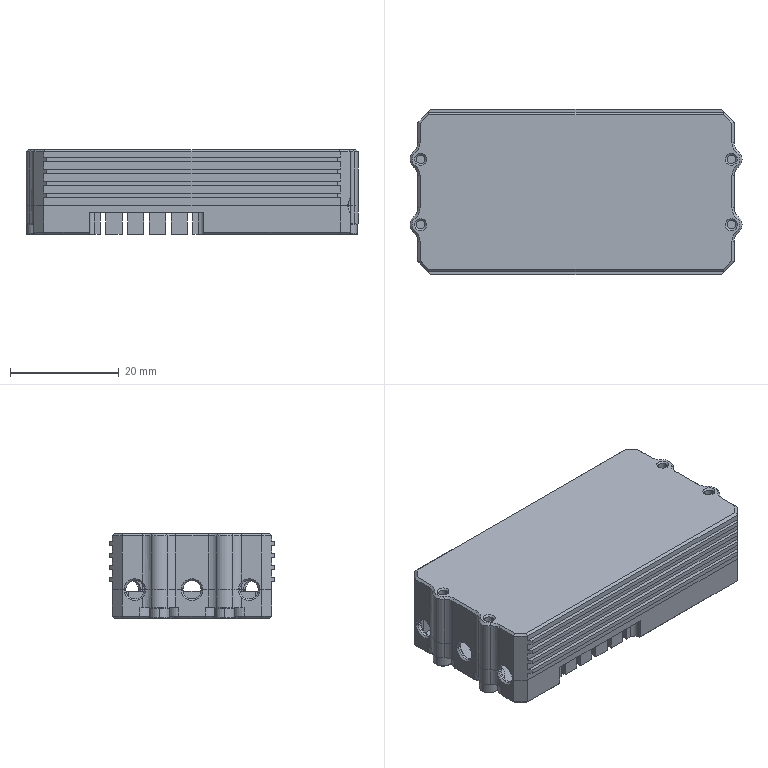Part | SolidWorks | features BaseBody 6 | 6 solids | 1045 faces | box 61 x 30.44 x 15.6 mm | volume 7234 mm3 | plane 448 | cylinder 393 | cone 116 | spline 72 | torus 16 | commonest cylinder face diameters 2.4 x128 4 x72 2 x33 0.157 x24 0.236 x24 3.9 x24